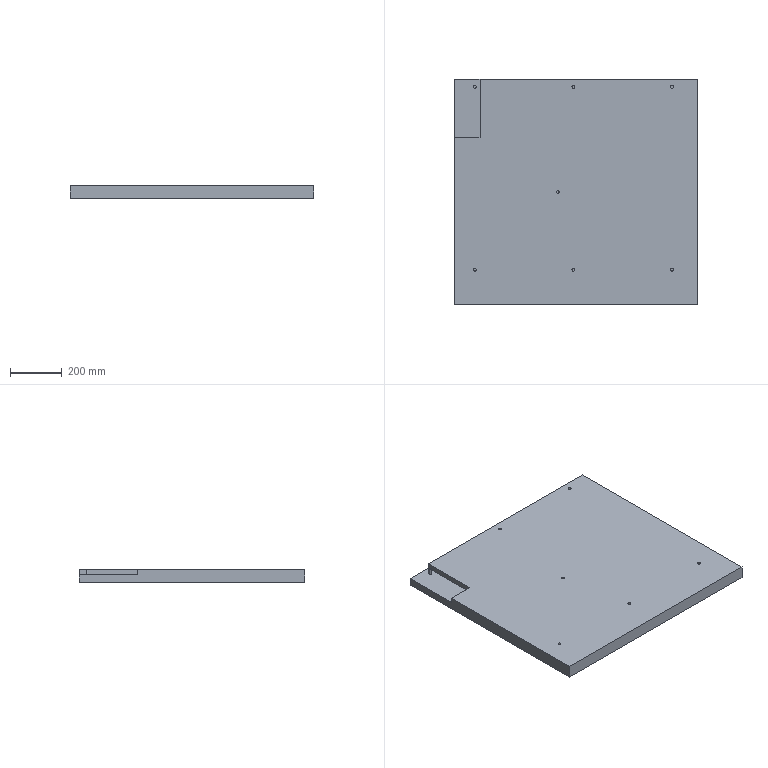Part | 1 solid | 30 faces | box 940 x 870 x 50 mm | volume 40430827 mm3 | plane 16 | cylinder 14 | commonest cylinder face diameters 11 x12 10 x2
STEP:
#1=CARTESIAN_POINT('',(-15.5,405.,30.));
#2=VERTEX_POINT('',#1);
#3=CARTESIAN_POINT('',(-4.5,405.,30.));
#4=VERTEX_POINT('',#3);
#5=CARTESIAN_POINT('',(-10.,405.,30.));
#6=DIRECTION('',(0.,0.,1.));
#7=DIRECTION('',(-1.,0.,0.));
#8=AXIS2_PLACEMENT_3D('',#5,#6,#7);
#9=CIRCLE('',#8,5.5);
#10=EDGE_CURVE('',#2,#4,#9,.T.);
#11=ORIENTED_EDGE('',*,*,#10,.F.);
#12=CARTESIAN_POINT('',(-15.5,405.,50.));
#13=VERTEX_POINT('',#12);
#14=CARTESIAN_POINT('',(-15.5,405.,30.));
#15=DIRECTION('',(0.,0.,1.));
#16=VECTOR('',#15,1000.);
#17=LINE('',#14,#16);
#18=EDGE_CURVE('',#2,#13,#17,.T.);
#19=ORIENTED_EDGE('',*,*,#18,.T.);
#20=CARTESIAN_POINT('',(-4.5,405.,50.));
#21=VERTEX_POINT('',#20);
#22=CARTESIAN_POINT('',(-10.,405.,50.));
#23=DIRECTION('',(0.,0.,1.));
#24=DIRECTION('',(-1.,0.,0.));
#25=AXIS2_PLACEMENT_3D('',#22,#23,#24);
#26=CIRCLE('',#25,5.5);
#27=EDGE_CURVE('',#13,#21,#26,.T.);
#28=ORIENTED_EDGE('',*,*,#27,.T.);
#29=CARTESIAN_POINT('',(-4.5,405.,30.));
#30=DIRECTION('',(0.,0.,1.));
#31=VECTOR('',#30,1000.);
#32=LINE('',#29,#31);
#33=EDGE_CURVE('',#4,#21,#32,.T.);
#34=ORIENTED_EDGE('',*,*,#33,.F.);
#35=EDGE_LOOP('',(#11,#19,#28,#34));
#36=FACE_OUTER_BOUND('',#35,.T.);
#37=CARTESIAN_POINT('',(-10.,405.,30.));
#38=DIRECTION('',(0.,0.,1.));
#39=DIRECTION('',(1.,0.,0.));
#40=AXIS2_PLACEMENT_3D('',#37,#38,#39);
#41=CYLINDRICAL_SURFACE('',#40,5.5);
#42=ADVANCED_FACE('',(#36),#41,.F.);
#43=CARTESIAN_POINT('',(364.5,405.,30.));
#44=VERTEX_POINT('',#43);
#45=CARTESIAN_POINT('',(375.5,405.,30.));
#46=VERTEX_POINT('',#45);
#47=CARTESIAN_POINT('',(370.,405.,30.));
#48=DIRECTION('',(0.,0.,1.));
#49=DIRECTION('',(-1.,0.,0.));
#50=AXIS2_PLACEMENT_3D('',#47,#48,#49);
#51=CIRCLE('',#50,5.5);
#52=EDGE_CURVE('',#44,#46,#51,.T.);
#53=ORIENTED_EDGE('',*,*,#52,.F.);
#54=CARTESIAN_POINT('',(364.5,405.,50.));
#55=VERTEX_POINT('',#54);
#56=CARTESIAN_POINT('',(364.5,405.,30.));
#57=DIRECTION('',(0.,0.,1.));
#58=VECTOR('',#57,1000.);
#59=LINE('',#56,#58);
#60=EDGE_CURVE('',#44,#55,#59,.T.);
#61=ORIENTED_EDGE('',*,*,#60,.T.);
#62=CARTESIAN_POINT('',(375.5,405.,50.));
#63=VERTEX_POINT('',#62);
#64=CARTESIAN_POINT('',(370.,405.,50.));
#65=DIRECTION('',(0.,0.,1.));
#66=DIRECTION('',(-1.,0.,0.));
#67=AXIS2_PLACEMENT_3D('',#64,#65,#66);
#68=CIRCLE('',#67,5.5);
#69=EDGE_CURVE('',#55,#63,#68,.T.);
#70=ORIENTED_EDGE('',*,*,#69,.T.);
#71=CARTESIAN_POINT('',(375.5,405.,30.));
#72=DIRECTION('',(0.,0.,1.));
#73=VECTOR('',#72,1000.);
#74=LINE('',#71,#73);
#75=EDGE_CURVE('',#46,#63,#74,.T.);
#76=ORIENTED_EDGE('',*,*,#75,.F.);
#77=EDGE_LOOP('',(#53,#61,#70,#76));
#78=FACE_OUTER_BOUND('',#77,.T.);
#79=CARTESIAN_POINT('',(370.,405.,30.));
#80=DIRECTION('',(0.,0.,1.));
#81=DIRECTION('',(1.,0.,0.));
#82=AXIS2_PLACEMENT_3D('',#79,#80,#81);
#83=CYLINDRICAL_SURFACE('',#82,5.5);
#84=ADVANCED_FACE('',(#78),#83,.F.);
#85=CARTESIAN_POINT('',(364.5,-300.,30.));
#86=VERTEX_POINT('',#85);
#87=CARTESIAN_POINT('',(375.5,-300.,30.));
#88=VERTEX_POINT('',#87);
#89=CARTESIAN_POINT('',(370.,-300.,30.));
#90=DIRECTION('',(0.,0.,1.));
#91=DIRECTION('',(1.,0.,0.));
#92=AXIS2_PLACEMENT_3D('',#89,#90,#91);
#93=CIRCLE('',#92,5.5);
#94=EDGE_CURVE('',#86,#88,#93,.T.);
#95=ORIENTED_EDGE('',*,*,#94,.F.);
#96=CARTESIAN_POINT('',(364.5,-300.,50.));
#97=VERTEX_POINT('',#96);
#98=CARTESIAN_POINT('',(364.5,-300.,30.));
#99=DIRECTION('',(0.,0.,1.));
#100=VECTOR('',#99,1000.);
#101=LINE('',#98,#100);
#102=EDGE_CURVE('',#86,#97,#101,.T.);
#103=ORIENTED_EDGE('',*,*,#102,.T.);
#104=CARTESIAN_POINT('',(375.5,-300.,50.));
#105=VERTEX_POINT('',#104);
#106=CARTESIAN_POINT('',(370.,-300.,50.));
#107=DIRECTION('',(0.,0.,1.));
#108=DIRECTION('',(1.,0.,0.));
#109=AXIS2_PLACEMENT_3D('',#106,#107,#108);
#110=CIRCLE('',#109,5.5);
#111=EDGE_CURVE('',#97,#105,#110,.T.);
#112=ORIENTED_EDGE('',*,*,#111,.T.);
#113=CARTESIAN_POINT('',(375.5,-300.,30.));
#114=DIRECTION('',(0.,0.,1.));
#115=VECTOR('',#114,1000.);
#116=LINE('',#113,#115);
#117=EDGE_CURVE('',#88,#105,#116,.T.);
#118=ORIENTED_EDGE('',*,*,#117,.F.);
#119=EDGE_LOOP('',(#95,#103,#112,#118));
#120=FACE_OUTER_BOUND('',#119,.T.);
#121=CARTESIAN_POINT('',(370.,-300.,30.));
#122=DIRECTION('',(0.,0.,1.));
#123=DIRECTION('',(1.,0.,0.));
#124=AXIS2_PLACEMENT_3D('',#121,#122,#123);
#125=CYLINDRICAL_SURFACE('',#124,5.5);
#126=ADVANCED_FACE('',(#120),#125,.F.);
#127=CARTESIAN_POINT('',(-15.5,-300.,30.));
#128=VERTEX_POINT('',#127);
#129=CARTESIAN_POINT('',(-4.5,-300.,30.));
#130=VERTEX_POINT('',#129);
#131=CARTESIAN_POINT('',(-10.,-300.,30.));
#132=DIRECTION('',(0.,0.,1.));
#133=DIRECTION('',(1.,0.,0.));
#134=AXIS2_PLACEMENT_3D('',#131,#132,#133);
#135=CIRCLE('',#134,5.5);
#136=EDGE_CURVE('',#128,#130,#135,.T.);
#137=ORIENTED_EDGE('',*,*,#136,.F.);
#138=CARTESIAN_POINT('',(-15.5,-300.,50.));
#139=VERTEX_POINT('',#138);
#140=CARTESIAN_POINT('',(-15.5,-300.,30.));
#141=DIRECTION('',(0.,0.,1.));
#142=VECTOR('',#141,1000.);
#143=LINE('',#140,#142);
#144=EDGE_CURVE('',#128,#139,#143,.T.);
#145=ORIENTED_EDGE('',*,*,#144,.T.);
#146=CARTESIAN_POINT('',(-4.5,-300.,50.));
#147=VERTEX_POINT('',#146);
#148=CARTESIAN_POINT('',(-10.,-300.,50.));
#149=DIRECTION('',(0.,0.,1.));
#150=DIRECTION('',(1.,0.,0.));
#151=AXIS2_PLACEMENT_3D('',#148,#149,#150);
#152=CIRCLE('',#151,5.5);
#153=EDGE_CURVE('',#139,#147,#152,.T.);
#154=ORIENTED_EDGE('',*,*,#153,.T.);
#155=CARTESIAN_POINT('',(-4.5,-300.,30.));
#156=DIRECTION('',(0.,0.,1.));
#157=VECTOR('',#156,1000.);
#158=LINE('',#155,#157);
#159=EDGE_CURVE('',#130,#147,#158,.T.);
#160=ORIENTED_EDGE('',*,*,#159,.F.);
#161=EDGE_LOOP('',(#137,#145,#154,#160));
#162=FACE_OUTER_BOUND('',#161,.T.);
#163=CARTESIAN_POINT('',(-10.,-300.,30.));
#164=DIRECTION('',(0.,0.,1.));
#165=DIRECTION('',(1.,0.,0.));
#166=AXIS2_PLACEMENT_3D('',#163,#164,#165);
#167=CYLINDRICAL_SURFACE('',#166,5.5);
#168=ADVANCED_FACE('',(#162),#167,.F.);
#169=CARTESIAN_POINT('',(-395.5,-300.,30.));
#170=VERTEX_POINT('',#169);
#171=CARTESIAN_POINT('',(-384.5,-300.,30.));
#172=VERTEX_POINT('',#171);
#173=CARTESIAN_POINT('',(-390.,-300.,30.));
#174=DIRECTION('',(0.,0.,1.));
#175=DIRECTION('',(1.,0.,0.));
#176=AXIS2_PLACEMENT_3D('',#173,#174,#175);
#177=CIRCLE('',#176,5.5);
#178=EDGE_CURVE('',#170,#172,#177,.T.);
#179=ORIENTED_EDGE('',*,*,#178,.F.);
#180=CARTESIAN_POINT('',(-395.5,-300.,50.));
#181=VERTEX_POINT('',#180);
#182=CARTESIAN_POINT('',(-395.5,-300.,30.));
#183=DIRECTION('',(0.,0.,1.));
#184=VECTOR('',#183,1000.);
#185=LINE('',#182,#184);
#186=EDGE_CURVE('',#170,#181,#185,.T.);
#187=ORIENTED_EDGE('',*,*,#186,.T.);
#188=CARTESIAN_POINT('',(-384.5,-300.,50.));
#189=VERTEX_POINT('',#188);
#190=CARTESIAN_POINT('',(-390.,-300.,50.));
#191=DIRECTION('',(0.,0.,1.));
#192=DIRECTION('',(1.,0.,0.));
#193=AXIS2_PLACEMENT_3D('',#190,#191,#192);
#194=CIRCLE('',#193,5.5);
#195=EDGE_CURVE('',#181,#189,#194,.T.);
#196=ORIENTED_EDGE('',*,*,#195,.T.);
#197=CARTESIAN_POINT('',(-384.5,-300.,30.));
#198=DIRECTION('',(0.,0.,1.));
#199=VECTOR('',#198,1000.);
#200=LINE('',#197,#199);
#201=EDGE_CURVE('',#172,#189,#200,.T.);
#202=ORIENTED_EDGE('',*,*,#201,.F.);
#203=EDGE_LOOP('',(#179,#187,#196,#202));
#204=FACE_OUTER_BOUND('',#203,.T.);
#205=CARTESIAN_POINT('',(-390.,-300.,30.));
#206=DIRECTION('',(0.,0.,1.));
#207=DIRECTION('',(1.,0.,0.));
#208=AXIS2_PLACEMENT_3D('',#205,#206,#207);
#209=CYLINDRICAL_SURFACE('',#208,5.5);
#210=ADVANCED_FACE('',(#204),#209,.F.);
#211=CARTESIAN_POINT('',(-75.,0.,30.));
#212=VERTEX_POINT('',#211);
#213=CARTESIAN_POINT('',(-65.,0.,30.));
#214=VERTEX_POINT('',#213);
#215=CARTESIAN_POINT('',(-70.,0.,30.));
#216=DIRECTION('',(0.,0.,1.));
#217=DIRECTION('',(1.,0.,0.));
#218=AXIS2_PLACEMENT_3D('',#215,#216,#217);
#219=CIRCLE('',#218,5.);
#220=EDGE_CURVE('',#212,#214,#219,.T.);
#221=ORIENTED_EDGE('',*,*,#220,.F.);
#222=CARTESIAN_POINT('',(-75.,0.,50.));
#223=VERTEX_POINT('',#222);
#224=CARTESIAN_POINT('',(-75.,0.,30.));
#225=DIRECTION('',(0.,0.,1.));
#226=VECTOR('',#225,1000.);
#227=LINE('',#224,#226);
#228=EDGE_CURVE('',#212,#223,#227,.T.);
#229=ORIENTED_EDGE('',*,*,#228,.T.);
#230=CARTESIAN_POINT('',(-65.,0.,50.));
#231=VERTEX_POINT('',#230);
#232=CARTESIAN_POINT('',(-70.,0.,50.));
#233=DIRECTION('',(0.,0.,1.));
#234=DIRECTION('',(1.,0.,0.));
#235=AXIS2_PLACEMENT_3D('',#232,#233,#234);
#236=CIRCLE('',#235,5.);
#237=EDGE_CURVE('',#223,#231,#236,.T.);
#238=ORIENTED_EDGE('',*,*,#237,.T.);
#239=CARTESIAN_POINT('',(-65.,0.,30.));
#240=DIRECTION('',(0.,0.,1.));
#241=VECTOR('',#240,1000.);
#242=LINE('',#239,#241);
#243=EDGE_CURVE('',#214,#231,#242,.T.);
#244=ORIENTED_EDGE('',*,*,#243,.F.);
#245=EDGE_LOOP('',(#221,#229,#238,#244));
#246=FACE_OUTER_BOUND('',#245,.T.);
#247=CARTESIAN_POINT('',(-70.,0.,30.));
#248=DIRECTION('',(0.,0.,1.));
#249=DIRECTION('',(1.,0.,0.));
#250=AXIS2_PLACEMENT_3D('',#247,#248,#249);
#251=CYLINDRICAL_SURFACE('',#250,5.);
#252=ADVANCED_FACE('',(#246),#251,.F.);
#253=CARTESIAN_POINT('',(-384.5,405.,30.));
#254=VERTEX_POINT('',#253);
#255=CARTESIAN_POINT('',(-395.5,405.,30.));
#256=VERTEX_POINT('',#255);
#257=CARTESIAN_POINT('',(-390.,405.,30.));
#258=DIRECTION('',(0.,0.,1.));
#259=DIRECTION('',(-1.,0.,0.));
#260=AXIS2_PLACEMENT_3D('',#257,#258,#259);
#261=CIRCLE('',#260,5.5);
#262=EDGE_CURVE('',#254,#256,#261,.T.);
#263=ORIENTED_EDGE('',*,*,#262,.T.);
#264=CARTESIAN_POINT('',(-395.5,405.,50.));
#265=VERTEX_POINT('',#264);
#266=CARTESIAN_POINT('',(-395.5,405.,30.));
#267=DIRECTION('',(0.,0.,1.));
#268=VECTOR('',#267,1000.);
#269=LINE('',#266,#268);
#270=EDGE_CURVE('',#256,#265,#269,.T.);
#271=ORIENTED_EDGE('',*,*,#270,.T.);
#272=CARTESIAN_POINT('',(-384.5,405.,50.));
#273=VERTEX_POINT('',#272);
#274=CARTESIAN_POINT('',(-390.,405.,50.));
#275=DIRECTION('',(0.,0.,1.));
#276=DIRECTION('',(-1.,0.,0.));
#277=AXIS2_PLACEMENT_3D('',#274,#275,#276);
#278=CIRCLE('',#277,5.5);
#279=EDGE_CURVE('',#273,#265,#278,.T.);
#280=ORIENTED_EDGE('',*,*,#279,.F.);
#281=CARTESIAN_POINT('',(-384.5,405.,30.));
#282=DIRECTION('',(0.,0.,1.));
#283=VECTOR('',#282,1000.);
#284=LINE('',#281,#283);
#285=EDGE_CURVE('',#254,#273,#284,.T.);
#286=ORIENTED_EDGE('',*,*,#285,.F.);
#287=EDGE_LOOP('',(#263,#271,#280,#286));
#288=FACE_OUTER_BOUND('',#287,.T.);
#289=CARTESIAN_POINT('',(-390.,405.,30.));
#290=DIRECTION('',(0.,0.,1.));
#291=DIRECTION('',(1.,0.,0.));
#292=AXIS2_PLACEMENT_3D('',#289,#290,#291);
#293=CYLINDRICAL_SURFACE('',#292,5.5);
#294=ADVANCED_FACE('',(#288),#293,.T.);
#295=CARTESIAN_POINT('',(470.,-435.,0.));
#296=VERTEX_POINT('',#295);
#297=CARTESIAN_POINT('',(470.,435.,0.));
#298=VERTEX_POINT('',#297);
#299=CARTESIAN_POINT('',(470.,435.,0.));
#300=DIRECTION('',(0.,1.,0.));
#301=VECTOR('',#300,1000.);
#302=LINE('',#299,#301);
#303=EDGE_CURVE('',#296,#298,#302,.T.);
#304=ORIENTED_EDGE('',*,*,#303,.T.);
#305=CARTESIAN_POINT('',(470.,435.,50.));
#306=VERTEX_POINT('',#305);
#307=CARTESIAN_POINT('',(470.,435.,50.));
#308=DIRECTION('',(0.,0.,-1.));
#309=VECTOR('',#308,1000.);
#310=LINE('',#307,#309);
#311=EDGE_CURVE('',#306,#298,#310,.T.);
#312=ORIENTED_EDGE('',*,*,#311,.F.);
#313=CARTESIAN_POINT('',(470.,-435.,50.));
#314=VERTEX_POINT('',#313);
#315=CARTESIAN_POINT('',(470.,435.,50.));
#316=DIRECTION('',(0.,1.,0.));
#317=VECTOR('',#316,1000.);
#318=LINE('',#315,#317);
#319=EDGE_CURVE('',#314,#306,#318,.T.);
#320=ORIENTED_EDGE('',*,*,#319,.F.);
#321=CARTESIAN_POINT('',(470.,-435.,50.));
#322=DIRECTION('',(0.,0.,-1.));
#323=VECTOR('',#322,1000.);
#324=LINE('',#321,#323);
#325=EDGE_CURVE('',#314,#296,#324,.T.);
#326=ORIENTED_EDGE('',*,*,#325,.T.);
#327=EDGE_LOOP('',(#304,#312,#320,#326));
#328=FACE_OUTER_BOUND('',#327,.T.);
#329=CARTESIAN_POINT('',(470.,435.,50.));
#330=DIRECTION('',(-1.,0.,0.));
#331=DIRECTION('',(0.,-1.,0.));
#332=AXIS2_PLACEMENT_3D('',#329,#330,#331);
#333=PLANE('',#332);
#334=ADVANCED_FACE('',(#328),#333,.F.);
#335=CARTESIAN_POINT('',(-370.,435.,30.));
#336=VERTEX_POINT('',#335);
#337=CARTESIAN_POINT('',(-470.,435.,30.));
#338=VERTEX_POINT('',#337);
#339=CARTESIAN_POINT('',(-470.,435.,30.));
#340=DIRECTION('',(-1.,0.,0.));
#341=VECTOR('',#340,1000.);
#342=LINE('',#339,#341);
#343=EDGE_CURVE('',#336,#338,#342,.T.);
#344=ORIENTED_EDGE('',*,*,#343,.F.);
#345=CARTESIAN_POINT('',(-370.,435.,50.));
#346=VERTEX_POINT('',#345);
#347=CARTESIAN_POINT('',(-370.,435.,50.));
#348=DIRECTION('',(0.,0.,1.));
#349=VECTOR('',#348,1000.);
#350=LINE('',#347,#349);
#351=EDGE_CURVE('',#336,#346,#350,.T.);
#352=ORIENTED_EDGE('',*,*,#351,.T.);
#353=CARTESIAN_POINT('',(-470.,435.,50.));
#354=DIRECTION('',(-1.,0.,0.));
#355=VECTOR('',#354,1000.);
#356=LINE('',#353,#355);
#357=EDGE_CURVE('',#306,#346,#356,.T.);
#358=ORIENTED_EDGE('',*,*,#357,.F.);
#359=ORIENTED_EDGE('',*,*,#311,.T.);
#360=CARTESIAN_POINT('',(-470.,435.,0.));
#361=VERTEX_POINT('',#360);
#362=CARTESIAN_POINT('',(-470.,435.,0.));
#363=DIRECTION('',(-1.,0.,0.));
#364=VECTOR('',#363,1000.);
#365=LINE('',#362,#364);
#366=EDGE_CURVE('',#298,#361,#365,.T.);
#367=ORIENTED_EDGE('',*,*,#366,.T.);
#368=CARTESIAN_POINT('',(-470.,435.,50.));
#369=DIRECTION('',(0.,0.,-1.));
#370=VECTOR('',#369,1000.);
#371=LINE('',#368,#370);
#372=EDGE_CURVE('',#338,#361,#371,.T.);
#373=ORIENTED_EDGE('',*,*,#372,.F.);
#374=EDGE_LOOP('',(#344,#352,#358,#359,#367,#373));
#375=FACE_OUTER_BOUND('',#374,.T.);
#376=CARTESIAN_POINT('',(-470.,435.,50.));
#377=DIRECTION('',(0.,-1.,0.));
#378=DIRECTION('',(0.,0.,-1.));
#379=AXIS2_PLACEMENT_3D('',#376,#377,#378);
#380=PLANE('',#379);
#381=ADVANCED_FACE('',(#375),#380,.F.);
#382=CARTESIAN_POINT('',(-470.,210.,50.));
#383=VERTEX_POINT('',#382);
#384=CARTESIAN_POINT('',(-470.,-435.,50.));
#385=VERTEX_POINT('',#384);
#386=CARTESIAN_POINT('',(-470.,435.,50.));
#387=DIRECTION('',(0.,-1.,0.));
#388=VECTOR('',#387,1000.);
#389=LINE('',#386,#388);
#390=EDGE_CURVE('',#383,#385,#389,.T.);
#391=ORIENTED_EDGE('',*,*,#390,.F.);
#392=CARTESIAN_POINT('',(-470.,210.,30.));
#393=VERTEX_POINT('',#392);
#394=CARTESIAN_POINT('',(-470.,210.,50.));
#395=DIRECTION('',(0.,0.,-1.));
#396=VECTOR('',#395,1000.);
#397=LINE('',#394,#396);
#398=EDGE_CURVE('',#383,#393,#397,.T.);
#399=ORIENTED_EDGE('',*,*,#398,.T.);
#400=CARTESIAN_POINT('',(-470.,435.,30.));
#401=DIRECTION('',(0.,-1.,0.));
#402=VECTOR('',#401,1000.);
#403=LINE('',#400,#402);
#404=EDGE_CURVE('',#338,#393,#403,.T.);
#405=ORIENTED_EDGE('',*,*,#404,.F.);
#406=ORIENTED_EDGE('',*,*,#372,.T.);
#407=CARTESIAN_POINT('',(-470.,-435.,0.));
#408=VERTEX_POINT('',#407);
#409=CARTESIAN_POINT('',(-470.,435.,0.));
#410=DIRECTION('',(0.,-1.,0.));
#411=VECTOR('',#410,1000.);
#412=LINE('',#409,#411);
#413=EDGE_CURVE('',#361,#408,#412,.T.);
#414=ORIENTED_EDGE('',*,*,#413,.T.);
#415=CARTESIAN_POINT('',(-470.,-435.,50.));
#416=DIRECTION('',(0.,0.,-1.));
#417=VECTOR('',#416,1000.);
#418=LINE('',#415,#417);
#419=EDGE_CURVE('',#385,#408,#418,.T.);
#420=ORIENTED_EDGE('',*,*,#419,.F.);
#421=EDGE_LOOP('',(#391,#399,#405,#406,#414,#420));
#422=FACE_OUTER_BOUND('',#421,.T.);
#423=CARTESIAN_POINT('',(-470.,435.,50.));
#424=DIRECTION('',(1.,0.,0.));
#425=DIRECTION('',(0.,1.,0.));
#426=AXIS2_PLACEMENT_3D('',#423,#424,#425);
#427=PLANE('',#426);
#428=ADVANCED_FACE('',(#422),#427,.F.);
#429=CARTESIAN_POINT('',(-470.,-435.,0.));
#430=DIRECTION('',(1.,0.,0.));
#431=VECTOR('',#430,1000.);
#432=LINE('',#429,#431);
#433=EDGE_CURVE('',#408,#296,#432,.T.);
#434=ORIENTED_EDGE('',*,*,#433,.T.);
#435=ORIENTED_EDGE('',*,*,#325,.F.);
#436=CARTESIAN_POINT('',(-470.,-435.,50.));
#437=DIRECTION('',(1.,0.,0.));
#438=VECTOR('',#437,1000.);
#439=LINE('',#436,#438);
#440=EDGE_CURVE('',#385,#314,#439,.T.);
#441=ORIENTED_EDGE('',*,*,#440,.F.);
#442=ORIENTED_EDGE('',*,*,#419,.T.);
#443=EDGE_LOOP('',(#434,#435,#441,#442));
#444=FACE_OUTER_BOUND('',#443,.T.);
#445=CARTESIAN_POINT('',(-470.,-435.,50.));
#446=DIRECTION('',(0.,1.,0.));
#447=DIRECTION('',(0.,0.,1.));
#448=AXIS2_PLACEMENT_3D('',#445,#446,#447);
#449=PLANE('',#448);
#450=ADVANCED_FACE('',(#444),#449,.F.);
#451=CARTESIAN_POINT('',(-10.,405.,50.));
#452=DIRECTION('',(0.,0.,1.));
#453=DIRECTION('',(-1.,0.,0.));
#454=AXIS2_PLACEMENT_3D('',#451,#452,#453);
#455=CIRCLE('',#454,5.5);
#456=EDGE_CURVE('',#21,#13,#455,.T.);
#457=ORIENTED_EDGE('',*,*,#456,.F.);
#458=ORIENTED_EDGE('',*,*,#27,.F.);
#459=EDGE_LOOP('',(#457,#458));
#460=FACE_BOUND('',#459,.T.);
#461=CARTESIAN_POINT('',(370.,405.,50.));
#462=DIRECTION('',(0.,0.,1.));
#463=DIRECTION('',(-1.,0.,0.));
#464=AXIS2_PLACEMENT_3D('',#461,#462,#463);
#465=CIRCLE('',#464,5.5);
#466=EDGE_CURVE('',#63,#55,#465,.T.);
#467=ORIENTED_EDGE('',*,*,#466,.F.);
#468=ORIENTED_EDGE('',*,*,#69,.F.);
#469=EDGE_LOOP('',(#467,#468));
#470=FACE_BOUND('',#469,.T.);
#471=CARTESIAN_POINT('',(370.,-300.,50.));
#472=DIRECTION('',(0.,0.,1.));
#473=DIRECTION('',(1.,0.,0.));
#474=AXIS2_PLACEMENT_3D('',#471,#472,#473);
#475=CIRCLE('',#474,5.5);
#476=EDGE_CURVE('',#105,#97,#475,.T.);
#477=ORIENTED_EDGE('',*,*,#476,.F.);
#478=ORIENTED_EDGE('',*,*,#111,.F.);
#479=EDGE_LOOP('',(#477,#478));
#480=FACE_BOUND('',#479,.T.);
#481=CARTESIAN_POINT('',(-10.,-300.,50.));
#482=DIRECTION('',(0.,0.,1.));
#483=DIRECTION('',(1.,0.,0.));
#484=AXIS2_PLACEMENT_3D('',#481,#482,#483);
#485=CIRCLE('',#484,5.5);
#486=EDGE_CURVE('',#147,#139,#485,.T.);
#487=ORIENTED_EDGE('',*,*,#486,.F.);
#488=ORIENTED_EDGE('',*,*,#153,.F.);
#489=EDGE_LOOP('',(#487,#488));
#490=FACE_BOUND('',#489,.T.);
#491=CARTESIAN_POINT('',(-390.,-300.,50.));
#492=DIRECTION('',(0.,0.,1.));
#493=DIRECTION('',(1.,0.,0.));
#494=AXIS2_PLACEMENT_3D('',#491,#492,#493);
#495=CIRCLE('',#494,5.5);
#496=EDGE_CURVE('',#189,#181,#495,.T.);
#497=ORIENTED_EDGE('',*,*,#496,.F.);
#498=ORIENTED_EDGE('',*,*,#195,.F.);
#499=EDGE_LOOP('',(#497,#498));
#500=FACE_BOUND('',#499,.T.);
#501=CARTESIAN_POINT('',(-70.,0.,50.));
#502=DIRECTION('',(0.,0.,1.));
#503=DIRECTION('',(1.,0.,0.));
#504=AXIS2_PLACEMENT_3D('',#501,#502,#503);
#505=CIRCLE('',#504,5.);
#506=EDGE_CURVE('',#231,#223,#505,.T.);
#507=ORIENTED_EDGE('',*,*,#506,.F.);
#508=ORIENTED_EDGE('',*,*,#237,.F.);
#509=EDGE_LOOP('',(#507,#508));
#510=FACE_BOUND('',#509,.T.);
#511=CARTESIAN_POINT('',(-370.,210.,50.));
#512=VERTEX_POINT('',#511);
#513=CARTESIAN_POINT('',(-370.,210.,50.));
#514=DIRECTION('',(0.,1.,0.));
#515=VECTOR('',#514,1000.);
#516=LINE('',#513,#515);
#517=EDGE_CURVE('',#512,#346,#516,.T.);
#518=ORIENTED_EDGE('',*,*,#517,.F.);
#519=CARTESIAN_POINT('',(0.,210.,50.));
#520=DIRECTION('',(1.,0.,0.));
#521=VECTOR('',#520,1000.);
#522=LINE('',#519,#521);
#523=EDGE_CURVE('',#383,#512,#522,.T.);
#524=ORIENTED_EDGE('',*,*,#523,.F.);
#525=ORIENTED_EDGE('',*,*,#390,.T.);
#526=ORIENTED_EDGE('',*,*,#440,.T.);
#527=ORIENTED_EDGE('',*,*,#319,.T.);
#528=ORIENTED_EDGE('',*,*,#357,.T.);
#529=EDGE_LOOP('',(#518,#524,#525,#526,#527,#528));
#530=FACE_OUTER_BOUND('',#529,.T.);
#531=CARTESIAN_POINT('',(0.,0.,50.));
#532=DIRECTION('',(0.,0.,1.));
#533=DIRECTION('',(1.,0.,0.));
#534=AXIS2_PLACEMENT_3D('',#531,#532,#533);
#535=PLANE('',#534);
#536=ADVANCED_FACE('',(#460,#470,#480,#490,#500,#510,#530),#535,.T.);
#537=ORIENTED_EDGE('',*,*,#303,.F.);
#538=ORIENTED_EDGE('',*,*,#433,.F.);
#539=ORIENTED_EDGE('',*,*,#413,.F.);
#540=ORIENTED_EDGE('',*,*,#366,.F.);
#541=EDGE_LOOP('',(#537,#538,#539,#540));
#542=FACE_OUTER_BOUND('',#541,.T.);
#543=CARTESIAN_POINT('',(0.,0.,0.));
#544=DIRECTION('',(0.,0.,1.));
#545=DIRECTION('',(1.,0.,0.));
#546=AXIS2_PLACEMENT_3D('',#543,#544,#545);
#547=PLANE('',#546);
#548=ADVANCED_FACE('',(#542),#547,.F.);
#549=ORIENTED_EDGE('',*,*,#262,.F.);
#550=CARTESIAN_POINT('',(-390.,405.,30.));
#551=DIRECTION('',(0.,0.,1.));
#552=DIRECTION('',(-1.,0.,0.));
#553=AXIS2_PLACEMENT_3D('',#550,#551,#552);
#554=CIRCLE('',#553,5.5);
#555=EDGE_CURVE('',#256,#254,#554,.T.);
#556=ORIENTED_EDGE('',*,*,#555,.F.);
#557=EDGE_LOOP('',(#549,#556));
#558=FACE_BOUND('',#557,.T.);
#559=ORIENTED_EDGE('',*,*,#343,.T.);
#560=ORIENTED_EDGE('',*,*,#404,.T.);
#561=CARTESIAN_POINT('',(-370.,210.,30.));
#562=VERTEX_POINT('',#561);
#563=CARTESIAN_POINT('',(-370.,210.,30.));
#564=DIRECTION('',(1.,0.,0.));
#565=VECTOR('',#564,1000.);
#566=LINE('',#563,#565);
#567=EDGE_CURVE('',#393,#562,#566,.T.);
#568=ORIENTED_EDGE('',*,*,#567,.T.);
#569=CARTESIAN_POINT('',(-370.,210.,30.));
#570=DIRECTION('',(0.,1.,0.));
#571=VECTOR('',#570,1000.);
#572=LINE('',#569,#571);
#573=EDGE_CURVE('',#562,#336,#572,.T.);
#574=ORIENTED_EDGE('',*,*,#573,.T.);
#575=EDGE_LOOP('',(#559,#560,#568,#574));
#576=FACE_OUTER_BOUND('',#575,.T.);
#577=CARTESIAN_POINT('',(0.,0.,30.));
#578=DIRECTION('',(0.,0.,1.));
#579=DIRECTION('',(1.,0.,0.));
#580=AXIS2_PLACEMENT_3D('',#577,#578,#579);
#581=PLANE('',#580);
#582=ADVANCED_FACE('',(#558,#576),#581,.T.);
#583=ORIENTED_EDGE('',*,*,#573,.F.);
#584=CARTESIAN_POINT('',(-370.,210.,30.));
#585=DIRECTION('',(0.,0.,1.));
#586=VECTOR('',#585,1000.);
#587=LINE('',#584,#586);
#588=EDGE_CURVE('',#562,#512,#587,.T.);
#589=ORIENTED_EDGE('',*,*,#588,.T.);
#590=ORIENTED_EDGE('',*,*,#517,.T.);
#591=ORIENTED_EDGE('',*,*,#351,.F.);
#592=EDGE_LOOP('',(#583,#589,#590,#591));
#593=FACE_OUTER_BOUND('',#592,.T.);
#594=CARTESIAN_POINT('',(-370.,210.,30.));
#595=DIRECTION('',(1.,0.,0.));
#596=DIRECTION('',(0.,0.,-1.));
#597=AXIS2_PLACEMENT_3D('',#594,#595,#596);
#598=PLANE('',#597);
#599=ADVANCED_FACE('',(#593),#598,.F.);
#600=ORIENTED_EDGE('',*,*,#523,.T.);
#601=ORIENTED_EDGE('',*,*,#588,.F.);
#602=ORIENTED_EDGE('',*,*,#567,.F.);
#603=ORIENTED_EDGE('',*,*,#398,.F.);
#604=EDGE_LOOP('',(#600,#601,#602,#603));
#605=FACE_OUTER_BOUND('',#604,.T.);
#606=CARTESIAN_POINT('',(-370.,210.,30.));
#607=DIRECTION('',(0.,-1.,0.));
#608=DIRECTION('',(0.,0.,-1.));
#609=AXIS2_PLACEMENT_3D('',#606,#607,#608);
#610=PLANE('',#609);
#611=ADVANCED_FACE('',(#605),#610,.F.);
#612=ORIENTED_EDGE('',*,*,#270,.F.);
#613=ORIENTED_EDGE('',*,*,#555,.T.);
#614=ORIENTED_EDGE('',*,*,#285,.T.);
#615=CARTESIAN_POINT('',(-390.,405.,50.));
#616=DIRECTION('',(0.,0.,1.));
#617=DIRECTION('',(-1.,0.,0.));
#618=AXIS2_PLACEMENT_3D('',#615,#616,#617);
#619=CIRCLE('',#618,5.5);
#620=EDGE_CURVE('',#265,#273,#619,.T.);
#621=ORIENTED_EDGE('',*,*,#620,.F.);
#622=EDGE_LOOP('',(#612,#613,#614,#621));
#623=FACE_OUTER_BOUND('',#622,.T.);
#624=CARTESIAN_POINT('',(-390.,405.,30.));
#625=DIRECTION('',(0.,0.,1.));
#626=DIRECTION('',(1.,0.,0.));
#627=AXIS2_PLACEMENT_3D('',#624,#625,#626);
#628=CYLINDRICAL_SURFACE('',#627,5.5);
#629=ADVANCED_FACE('',(#623),#628,.T.);
#630=ORIENTED_EDGE('',*,*,#228,.F.);
#631=CARTESIAN_POINT('',(-70.,0.,30.));
#632=DIRECTION('',(0.,0.,1.));
#633=DIRECTION('',(1.,0.,0.));
#634=AXIS2_PLACEMENT_3D('',#631,#632,#633);
#635=CIRCLE('',#634,5.);
#636=EDGE_CURVE('',#214,#212,#635,.T.);
#637=ORIENTED_EDGE('',*,*,#636,.F.);
#638=ORIENTED_EDGE('',*,*,#243,.T.);
#639=ORIENTED_EDGE('',*,*,#506,.T.);
#640=EDGE_LOOP('',(#630,#637,#638,#639));
#641=FACE_OUTER_BOUND('',#640,.T.);
#642=CARTESIAN_POINT('',(-70.,0.,30.));
#643=DIRECTION('',(0.,0.,1.));
#644=DIRECTION('',(1.,0.,0.));
#645=AXIS2_PLACEMENT_3D('',#642,#643,#644);
#646=CYLINDRICAL_SURFACE('',#645,5.);
#647=ADVANCED_FACE('',(#641),#646,.F.);
#648=ORIENTED_EDGE('',*,*,#636,.T.);
#649=ORIENTED_EDGE('',*,*,#220,.T.);
#650=EDGE_LOOP('',(#648,#649));
#651=FACE_OUTER_BOUND('',#650,.T.);
#652=CARTESIAN_POINT('',(-70.,0.,30.));
#653=DIRECTION('',(0.,0.,1.));
#654=DIRECTION('',(1.,0.,0.));
#655=AXIS2_PLACEMENT_3D('',#652,#653,#654);
#656=PLANE('',#655);
#657=ADVANCED_FACE('',(#651),#656,.T.);
#658=ORIENTED_EDGE('',*,*,#186,.F.);
#659=CARTESIAN_POINT('',(-390.,-300.,30.));
#660=DIRECTION('',(0.,0.,1.));
#661=DIRECTION('',(1.,0.,0.));
#662=AXIS2_PLACEMENT_3D('',#659,#660,#661);
#663=CIRCLE('',#662,5.5);
#664=EDGE_CURVE('',#172,#170,#663,.T.);
#665=ORIENTED_EDGE('',*,*,#664,.F.);
#666=ORIENTED_EDGE('',*,*,#201,.T.);
#667=ORIENTED_EDGE('',*,*,#496,.T.);
#668=EDGE_LOOP('',(#658,#665,#666,#667));
#669=FACE_OUTER_BOUND('',#668,.T.);
#670=CARTESIAN_POINT('',(-390.,-300.,30.));
#671=DIRECTION('',(0.,0.,1.));
#672=DIRECTION('',(1.,0.,0.));
#673=AXIS2_PLACEMENT_3D('',#670,#671,#672);
#674=CYLINDRICAL_SURFACE('',#673,5.5);
#675=ADVANCED_FACE('',(#669),#674,.F.);
#676=ORIENTED_EDGE('',*,*,#664,.T.);
#677=ORIENTED_EDGE('',*,*,#178,.T.);
#678=EDGE_LOOP('',(#676,#677));
#679=FACE_OUTER_BOUND('',#678,.T.);
#680=CARTESIAN_POINT('',(-390.,-300.,30.));
#681=DIRECTION('',(0.,0.,1.));
#682=DIRECTION('',(1.,0.,0.));
#683=AXIS2_PLACEMENT_3D('',#680,#681,#682);
#684=PLANE('',#683);
#685=ADVANCED_FACE('',(#679),#684,.T.);
#686=ORIENTED_EDGE('',*,*,#144,.F.);
#687=CARTESIAN_POINT('',(-10.,-300.,30.));
#688=DIRECTION('',(0.,0.,1.));
#689=DIRECTION('',(1.,0.,0.));
#690=AXIS2_PLACEMENT_3D('',#687,#688,#689);
#691=CIRCLE('',#690,5.5);
#692=EDGE_CURVE('',#130,#128,#691,.T.);
#693=ORIENTED_EDGE('',*,*,#692,.F.);
#694=ORIENTED_EDGE('',*,*,#159,.T.);
#695=ORIENTED_EDGE('',*,*,#486,.T.);
#696=EDGE_LOOP('',(#686,#693,#694,#695));
#697=FACE_OUTER_BOUND('',#696,.T.);
#698=CARTESIAN_POINT('',(-10.,-300.,30.));
#699=DIRECTION('',(0.,0.,1.));
#700=DIRECTION('',(1.,0.,0.));
#701=AXIS2_PLACEMENT_3D('',#698,#699,#700);
#702=CYLINDRICAL_SURFACE('',#701,5.5);
#703=ADVANCED_FACE('',(#697),#702,.F.);
#704=ORIENTED_EDGE('',*,*,#692,.T.);
#705=ORIENTED_EDGE('',*,*,#136,.T.);
#706=EDGE_LOOP('',(#704,#705));
#707=FACE_OUTER_BOUND('',#706,.T.);
#708=CARTESIAN_POINT('',(-10.,-300.,30.));
#709=DIRECTION('',(0.,0.,1.));
#710=DIRECTION('',(1.,0.,0.));
#711=AXIS2_PLACEMENT_3D('',#708,#709,#710);
#712=PLANE('',#711);
#713=ADVANCED_FACE('',(#707),#712,.T.);
#714=ORIENTED_EDGE('',*,*,#102,.F.);
#715=CARTESIAN_POINT('',(370.,-300.,30.));
#716=DIRECTION('',(0.,0.,1.));
#717=DIRECTION('',(1.,0.,0.));
#718=AXIS2_PLACEMENT_3D('',#715,#716,#717);
#719=CIRCLE('',#718,5.5);
#720=EDGE_CURVE('',#88,#86,#719,.T.);
#721=ORIENTED_EDGE('',*,*,#720,.F.);
#722=ORIENTED_EDGE('',*,*,#117,.T.);
#723=ORIENTED_EDGE('',*,*,#476,.T.);
#724=EDGE_LOOP('',(#714,#721,#722,#723));
#725=FACE_OUTER_BOUND('',#724,.T.);
#726=CARTESIAN_POINT('',(370.,-300.,30.));
#727=DIRECTION('',(0.,0.,1.));
#728=DIRECTION('',(1.,0.,0.));
#729=AXIS2_PLACEMENT_3D('',#726,#727,#728);
#730=CYLINDRICAL_SURFACE('',#729,5.5);
#731=ADVANCED_FACE('',(#725),#730,.F.);
#732=ORIENTED_EDGE('',*,*,#720,.T.);
#733=ORIENTED_EDGE('',*,*,#94,.T.);
#734=EDGE_LOOP('',(#732,#733));
#735=FACE_OUTER_BOUND('',#734,.T.);
#736=CARTESIAN_POINT('',(370.,-300.,30.));
#737=DIRECTION('',(0.,0.,1.));
#738=DIRECTION('',(1.,0.,0.));
#739=AXIS2_PLACEMENT_3D('',#736,#737,#738);
#740=PLANE('',#739);
#741=ADVANCED_FACE('',(#735),#740,.T.);
#742=ORIENTED_EDGE('',*,*,#60,.F.);
#743=CARTESIAN_POINT('',(370.,405.,30.));
#744=DIRECTION('',(0.,0.,1.));
#745=DIRECTION('',(-1.,0.,0.));
#746=AXIS2_PLACEMENT_3D('',#743,#744,#745);
#747=CIRCLE('',#746,5.5);
#748=EDGE_CURVE('',#46,#44,#747,.T.);
#749=ORIENTED_EDGE('',*,*,#748,.F.);
#750=ORIENTED_EDGE('',*,*,#75,.T.);
#751=ORIENTED_EDGE('',*,*,#466,.T.);
#752=EDGE_LOOP('',(#742,#749,#750,#751));
#753=FACE_OUTER_BOUND('',#752,.T.);
#754=CARTESIAN_POINT('',(370.,405.,30.));
#755=DIRECTION('',(0.,0.,1.));
#756=DIRECTION('',(1.,0.,0.));
#757=AXIS2_PLACEMENT_3D('',#754,#755,#756);
#758=CYLINDRICAL_SURFACE('',#757,5.5);
#759=ADVANCED_FACE('',(#753),#758,.F.);
#760=ORIENTED_EDGE('',*,*,#748,.T.);
#761=ORIENTED_EDGE('',*,*,#52,.T.);
#762=EDGE_LOOP('',(#760,#761));
#763=FACE_OUTER_BOUND('',#762,.T.);
#764=CARTESIAN_POINT('',(370.,405.,30.));
#765=DIRECTION('',(0.,0.,-1.));
#766=DIRECTION('',(-1.,0.,0.));
#767=AXIS2_PLACEMENT_3D('',#764,#765,#766);
#768=PLANE('',#767);
#769=ADVANCED_FACE('',(#763),#768,.F.);
#770=ORIENTED_EDGE('',*,*,#18,.F.);
#771=CARTESIAN_POINT('',(-10.,405.,30.));
#772=DIRECTION('',(0.,0.,1.));
#773=DIRECTION('',(-1.,0.,0.));
#774=AXIS2_PLACEMENT_3D('',#771,#772,#773);
#775=CIRCLE('',#774,5.5);
#776=EDGE_CURVE('',#4,#2,#775,.T.);
#777=ORIENTED_EDGE('',*,*,#776,.F.);
#778=ORIENTED_EDGE('',*,*,#33,.T.);
#779=ORIENTED_EDGE('',*,*,#456,.T.);
#780=EDGE_LOOP('',(#770,#777,#778,#779));
#781=FACE_OUTER_BOUND('',#780,.T.);
#782=CARTESIAN_POINT('',(-10.,405.,30.));
#783=DIRECTION('',(0.,0.,1.));
#784=DIRECTION('',(1.,0.,0.));
#785=AXIS2_PLACEMENT_3D('',#782,#783,#784);
#786=CYLINDRICAL_SURFACE('',#785,5.5);
#787=ADVANCED_FACE('',(#781),#786,.F.);
#788=ORIENTED_EDGE('',*,*,#776,.T.);
#789=ORIENTED_EDGE('',*,*,#10,.T.);
#790=EDGE_LOOP('',(#788,#789));
#791=FACE_OUTER_BOUND('',#790,.T.);
#792=CARTESIAN_POINT('',(-10.,405.,30.));
#793=DIRECTION('',(0.,0.,-1.));
#794=DIRECTION('',(-1.,0.,0.));
#795=AXIS2_PLACEMENT_3D('',#792,#793,#794);
#796=PLANE('',#795);
#797=ADVANCED_FACE('',(#791),#796,.F.);
#798=ORIENTED_EDGE('',*,*,#279,.T.);
#799=ORIENTED_EDGE('',*,*,#620,.T.);
#800=EDGE_LOOP('',(#798,#799));
#801=FACE_OUTER_BOUND('',#800,.T.);
#802=CARTESIAN_POINT('',(0.,0.,50.));
#803=DIRECTION('',(0.,0.,1.));
#804=DIRECTION('',(1.,0.,0.));
#805=AXIS2_PLACEMENT_3D('',#802,#803,#804);
#806=PLANE('',#805);
#807=ADVANCED_FACE('',(#801),#806,.T.);
#808=CLOSED_SHELL('',(#42,#84,#126,#168,#210,#252,#294,#334,#381,#428,#450,#536,#548,#582,#599,#611,#629,#647,#657,#675,#685,#703,#713,#731,#741,#759,#769,#787,#797,#807));
#809=MANIFOLD_SOLID_BREP('',#808);
#810=CARTESIAN_POINT('',(0.,0.,0.));
#811=DIRECTION('',(0.,0.,1.));
#812=DIRECTION('',(1.,0.,0.));
#813=AXIS2_PLACEMENT_3D('',#810,#811,#812);
#814=(LENGTH_UNIT()NAMED_UNIT(*)SI_UNIT(.MILLI.,.METRE.));
#815=UNCERTAINTY_MEASURE_WITH_UNIT(LENGTH_MEASURE(0.00001),#814,'','');
#816=(NAMED_UNIT(*)PLANE_ANGLE_UNIT()SI_UNIT($,.RADIAN.));
#817=(NAMED_UNIT(*)SI_UNIT($,.STERADIAN.)SOLID_ANGLE_UNIT());
#818=(GEOMETRIC_REPRESENTATION_CONTEXT(3)GLOBAL_UNCERTAINTY_ASSIGNED_CONTEXT((#815))GLOBAL_UNIT_ASSIGNED_CONTEXT((#814,#816,#817))REPRESENTATION_CONTEXT('',''));
#819=ADVANCED_BREP_SHAPE_REPRESENTATION('',(#809,#813),#818);